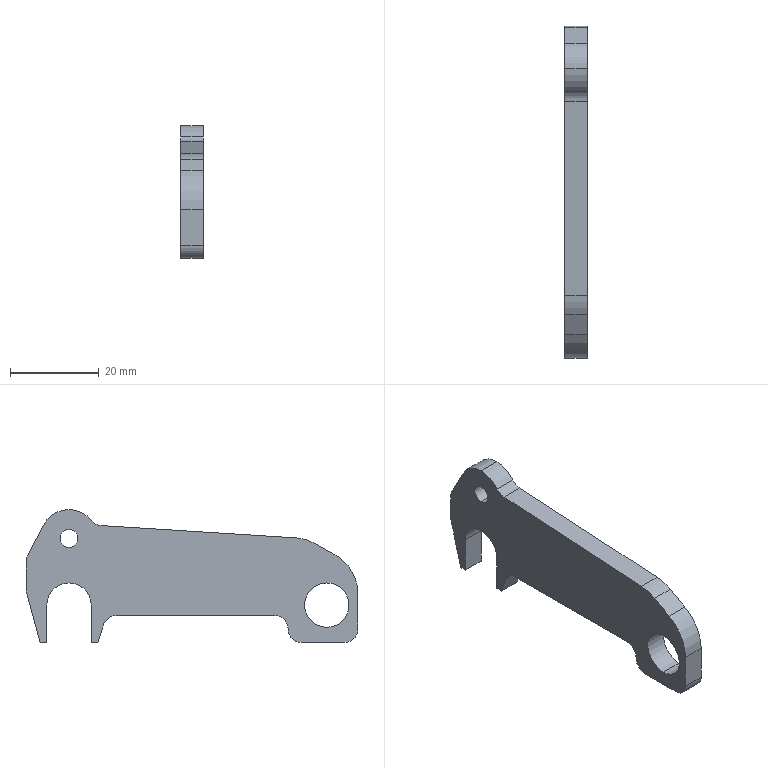Part | STEP file | Deraillieur Mount Brkt | 1 solid | 33 faces | box 5 x 74.673 x 29.884 mm | volume 6738 mm3 | cylinder 17 | plane 16 | commonest cylinder face diameters 6 x7 10 x4 4 x2 12.991 x2 20 x2